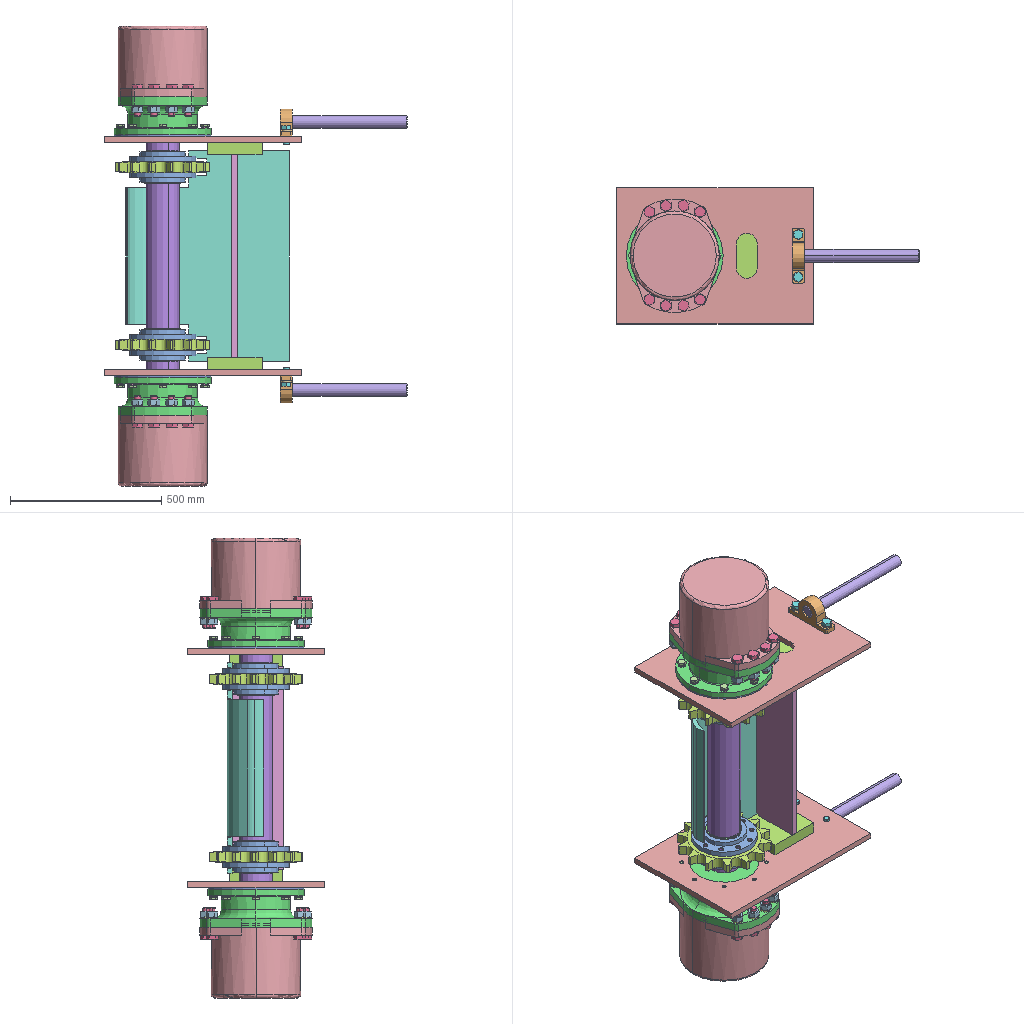Assembly | SolidWorks | 22 different items | 139 placed | box 1000 x 450 x 1519 mm
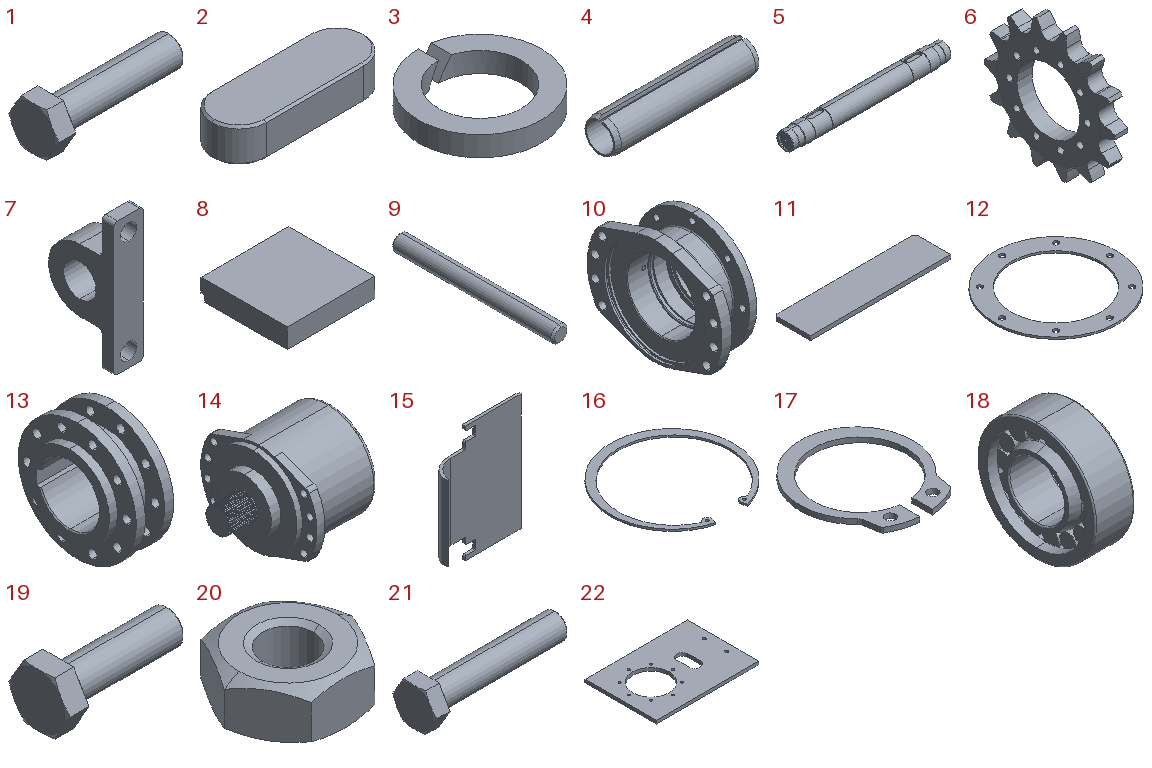Parts list (item | quantity | size | volume | features):
1 | x4 | 92.715 x 34.26 x 29.67 mm | 34696 mm3 | features RevCut 3, Boss 1, Chamfer 1, Extrusion 1, Fillet 1, LPattern 1
2 | x2 | 45 x 16 x 10 mm | 6612 mm3 | features Boss 2, Chamfer 1, Extrusion 1
3 | x36 | 19.1 x 19.1 x 3.1 mm | 465.776 mm3 | features Cut 1, Extrusion 1
4 | x20 | 70 x 16 x 15.922 mm | 4487 mm3 | features Boss 1, Cut 1, Extrusion 1, RevCut 1
5 | x1 | 948 x 110 x 110 mm | 7904078 mm3 | features Chamfer 2, ICE 2, Fillet 1, MirrorSolid 1, Revolution 1
6 | x2 | 36 x 312 x 306.035 mm | 1353964 mm3 | features ICE 2, CirPattern 1, Revolution 1
7 | x2 | 40 x 88.5 x 180 mm | 257790 mm3 | features Extrusion 1, Fillet 1, ICE 1
8 | x2 | 180 x 176 x 40 mm | 1249920 mm3 | features FlatPattern 1, ICE 1, SMBaseFlange 1, SheetMetal 1
9 | x2 | 42 x 420 x 42 mm | 579802 mm3 | features Chamfer 2, Extrusion 1
10 | x2 | 145 x 375 x 320 mm | 3842177 mm3 | features ICE 2, 3DProfileFeature 1, CirPattern 1, HoleWzd 1, Revolution 1
11 | x1 | 672 x 170 x 20 mm | 2281920 mm3 | features Chamfer 1, FlatPattern 1, SMBaseFlange 1, SheetMetal 1
12 | x2 | 320 x 320 x 5 mm | 188229 mm3 | features CirPattern 1, FlatPattern 1, HoleWzd 1, SMBaseFlange 1, SheetMetal 1
13 | x2 | 100 x 220 x 220 mm | 1419189 mm3 | features ICE 2, CirPattern 1, Revolution 1
14 | x2 | 366 x 375 x 295 mm | 18545806 mm3 | features ICE 2, RevCut 1, Revolution 1
15 | x1 | 540.8 x 120 x 696 mm | 5367152 mm3 | features ICE 2, Extrusion 1
16 | x2 | 189.5 x 186.271 x 3 mm | 15737 mm3 | features Extrusion 1
17 | x4 | 22.5 x 25.161 x 1 mm | 153.893 mm3 | features Fillet 2, Extrusion 1
18 | x2 | 114 x 340 x 340 mm | 5597424 mm3 | features Revolution 3, Fillet 2, CirPattern 1
19 | x16 | 19.5 x 9.238 x 8 mm | 500.222 mm3 | features RevCut 3, Boss 1, Chamfer 1, Extrusion 1, Fillet 1, LPattern 1
20 | x16 | 8.083 x 7 x 3.2 mm | 104.299 mm3 | features RevCut 2, Chamfer 1, Extrusion 1, LPattern 1
21 | x16 | 67.5 x 20.785 x 18 mm | 8849 mm3 | features RevCut 3, Boss 1, Chamfer 1, Extrusion 1, Fillet 1, LPattern 1
22 | x2 | 650 x 450 x 20 mm | 4798629 mm3 | features HoleWzd 3, CirPattern 2, FlatPattern 1, SMBaseFlange 1, SheetMetal 1
Mates (type | each side: item.copy, entity, surface, feature):
Coincident | 22.1 face plane Base-Flange1 | 8.1 face plane Base-Flange1
Coincident | 22.1 face plane Base-Flange1 | 12.1 face plane Base-Flange1
Coincident | 3.1 face plane Base-Extrude | 1.1 face plane BaseHead
Concentric | 22.1 face cylinder Base-Flange1 | 12.1 face cylinder Base-Flange1
DistanceDim | 8.1 face plane Base-Flange1 | 22.1 face plane Base-Flange1
DistanceDim | 22.1 face plane Base-Flange1 | 8.1 face plane Base-Flange1
Coincident | 7.1 face plane Boss-Extrude1 | 3.1 face plane Base-Extrude
Coincident | 8.1 face plane Base-Flange1 | 11.1 face plane Base-Flange1
Coincident | 8.1 face plane Cut-Extrude1 | 11.1 face plane Base-Flange1
Coincident | 8.1 face plane Cut-Extrude1 | 15.1 face plane Boss-Extrude1 | 2 times
Width | 11.1 face plane Base-Flange1 | 11.1 face plane Base-Flange1 | 8.1 face plane Base-Flange1 | 8.1 face plane Base-Flange1
DistanceDim | 22.1 face plane Base-Flange1 | 15.1 face plane Boss-Extrude1
Coincident | 22.2 face plane Base-Flange1 | 7.1 face plane Boss-Extrude1
Concentric | 22.2 face cylinder M20 Tapped Hole1 | 7.1 face cylinder Boss-Extrude1 | 2 times
Coincident | 7.1 face plane Boss-Extrude1 | 9.1 face plane Boss-Extrude1
Concentric | 7.1 face cylinder Boss-Extrude2 | 9.1 face cylinder Boss-Extrude1
Concentric | 3.1 face cylinder Base-Extrude | 1.1 face cylinder BaseBody
Concentric | 7.1 face cylinder Boss-Extrude1 | 1.1 face cylinder BaseBody
Concentric | 3.2 face cylinder Base-Extrude | 1.2 face cylinder BaseBody
Coincident | 3.2 face plane Base-Extrude | 1.2 face plane BaseHead
Coincident | 7.1 face plane Boss-Extrude1 | 3.2 face plane Base-Extrude
Concentric | 7.1 face cylinder Boss-Extrude1 | 1.2 face cylinder BaseBody
Concentric | 22.2 face cylinder Base-Flange1 | 5.1 face cylinder Revolve1
Concentric | 22.1 face cylinder M16 Tapped Hole2 | 12.1 face cylinder M16 Tapped Hole1
Concentric | 3.3 face cylinder Base-Extrude | 19.1 face cylinder BaseBody
Coincident | 3.3 face plane Base-Extrude | 19.1 face plane BaseHead
Concentric | 12.1 face cylinder Base-Flange1 | 10.1 face cylinder Revolve1
Concentric | 10.1 face cylinder CirPattern1 | 22.1 face cylinder CirPattern1
Coincident | 12.1 face plane Base-Flange1 | 10.1 face plane Revolve1
Concentric | 19.1 face cylinder BaseBody | 10.1 face cylinder Cut-Extrude2
Coincident | 3.3 face plane Base-Extrude | 10.1 face plane Revolve1
Concentric | 5.1 face cylinder Revolve1 | 18.1 face cylinder Revolve1
Coincident | 5.1 face plane Revolve1 | 18.1 face plane Revolve1
Concentric | 5.1 face cylinder Revolve1 | 16.1 face cylinder Body
Coincident | 10.1 face plane Revolve1 | 16.1 face plane Body
Concentric | 5.1 face cylinder Revolve1 | 14.1 face cylinder Revolve1
Concentric | 10.1 face cylinder Cut-Extrude1 | 14.1 face cylinder Cut-Extrude1
Coincident | 10.1 face plane Revolve1 | 14.1 face plane Revolve1
Coincident | 5.1 face plane Cut-Extrude1 | 2.1 face plane BaseKey | 2 times
Concentric | 5.1 face cylinder Cut-Extrude1 | 2.1 face cylinder BaseKey
Concentric | 5.1 face cylinder Revolve1 | 13.1 face cylinder Revolve1
Coincident | 2.1 face plane BaseKey | 13.1 face plane Cut-Extrude2
Width | 13.1 face plane Revolve1 | 13.1 face plane Revolve1 | assembly face | assembly face
Width | 13.1 face plane Revolve1 | 13.1 face plane Revolve1 | 5.1 face plane Revolve1 | 5.1 face plane Revolve1
Concentric | assembly face | 13.1 face cylinder CirPattern1
Concentric | 13.1 face cylinder Revolve1 | 6.1 face cylinder Revolve1
Concentric | 13.1 face cylinder CirPattern1 | 6.1 face cylinder CirPattern1
Width | 6.1 face plane Revolve1 | 6.1 face plane Revolve1 | 13.1 face plane Revolve1 | 13.1 face plane Revolve1
Coincident | 5.1 face plane Revolve1 | 17.1 face plane Body
Concentric | 5.1 face cylinder Revolve1 | 17.1 face cylinder Body
Coincident | 5.1 face plane Revolve1 | 17.2 face plane Body
Concentric | 5.1 face cylinder Revolve1 | 17.2 face cylinder Body
Coincident | 10.1 face plane Revolve1 | 18.1 face plane Revolve3
Concentric | 20.1 face cylinder BaseNut | 3.4 face cylinder Base-Extrude
Concentric | 21.1 face cylinder BaseBody | 3.4 face cylinder Base-Extrude
Coincident | 20.1 face plane BaseNut | 3.4 face plane Base-Extrude
Coincident | 10.2 face plane Revolve1 | 3.4 face plane Base-Extrude
Concentric | 14.2 face cylinder Cut-Extrude1 | 3.4 face cylinder Base-Extrude
Coincident | 14.2 face plane Revolve1 | 21.1 face plane BaseHead
Concentric | 20.2 face cylinder BaseNut | 3.5 face cylinder Base-Extrude
Concentric | 3.6 face cylinder Base-Extrude | 21.2 face cylinder BaseBody
Concentric | 20.3 face cylinder BaseNut | 3.7 face cylinder Base-Extrude
Concentric | 20.4 face cylinder BaseNut | 21.2 face cylinder BaseBody
Coincident | 20.4 face plane BaseNut | 3.6 face plane Base-Extrude
Coincident | 20.2 face plane BaseNut | 3.5 face plane Base-Extrude
Coincident | 20.3 face plane BaseNut | 3.7 face plane Base-Extrude
Concentric | 14.2 face cylinder Cut-Extrude1 | 3.6 face cylinder Base-Extrude
Coincident | 10.2 face plane Revolve1 | 3.6 face plane Base-Extrude
Coincident | 14.2 face plane Revolve1 | 21.2 face plane BaseHead
Coincident | 10.2 face plane Revolve1 | 3.7 face plane Base-Extrude
Concentric | 14.2 face cylinder Cut-Extrude1 | 3.7 face cylinder Base-Extrude
Concentric | 14.2 face cylinder Cut-Extrude1 | 3.5 face cylinder Base-Extrude
Coincident | 10.2 face plane Revolve1 | 3.5 face plane Base-Extrude
Concentric | 14.2 face cylinder Cut-Extrude1 | 21.3 face cylinder BaseBody
Coincident | 14.2 face plane Revolve1 | 21.3 face plane BaseHead
Concentric | 14.2 face cylinder Cut-Extrude1 | 21.4 face cylinder BaseBody
Coincident | 14.2 face plane Revolve1 | 21.4 face plane BaseHead
Concentric | 13.2 face cylinder Cut-Extrude1 | 4.1 face cylinder Base-Extrude
Coincident | 13.2 face plane Revolve1 | 4.1 face plane Base-Extrude
Concentric | 13.1 face cylinder Cut-Extrude1 | 4.2 face cylinder Base-Extrude
Coincident | 13.1 face plane Revolve1 | 4.2 face plane Base-Extrude